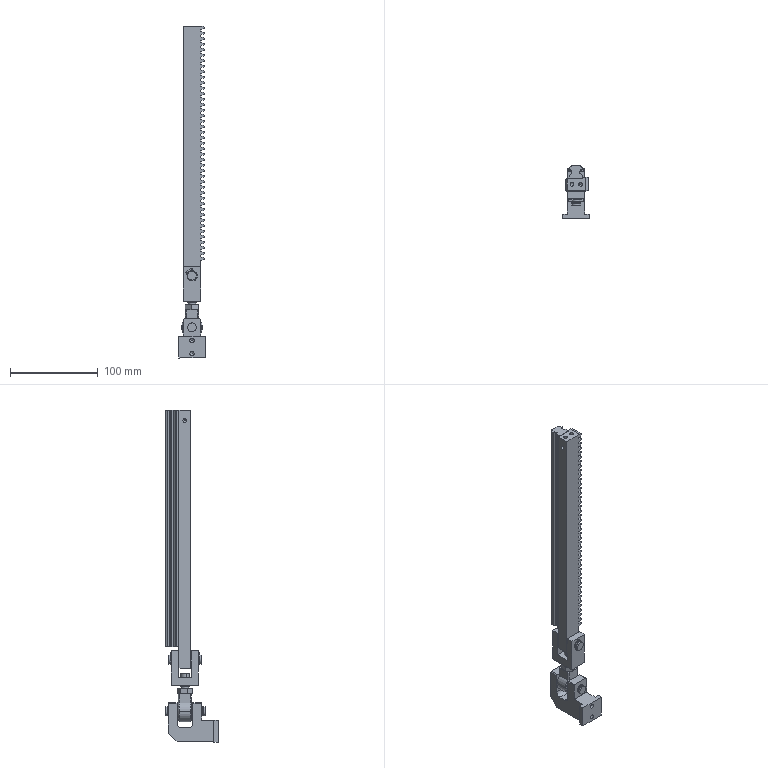Part | SolidWorks | 14 solids | 542 faces | box 30 x 59.858 x 379 mm | volume 198364 mm3 | plane 344 | cylinder 149 | cone 41 | torus 8 | commonest cylinder face diameters 10 x30 4.2 x10 0.8 x8 1.5 x8 3.3 x8 4 x8